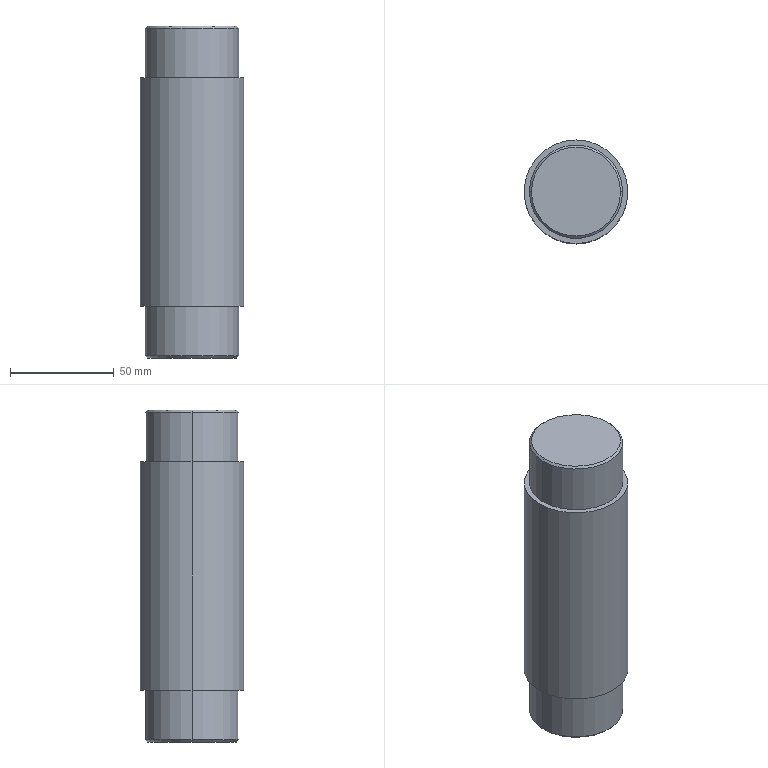Part | SolidWorks | features ICE 2, Chamfer 1, Extrusion 1 | 1 solid | 14 faces | box 50 x 50 x 160 mm | volume 295367 mm3 | cylinder 6 | cone 4 | plane 4 | commonest cylinder face diameters 45 x4 50 x2
STEP:
#1=CARTESIAN_POINT('',(-21.5,0.,-80.));
#2=VERTEX_POINT('',#1);
#3=CARTESIAN_POINT('',(21.5,0.,-80.));
#4=VERTEX_POINT('',#3);
#5=CARTESIAN_POINT('',(0.,0.,-80.));
#6=DIRECTION('',(0.,0.,-1.));
#7=DIRECTION('',(-1.,0.,0.));
#8=AXIS2_PLACEMENT_3D('',#5,#6,#7);
#9=CIRCLE('',#8,21.5);
#10=EDGE_CURVE('',#2,#4,#9,.T.);
#11=ORIENTED_EDGE('',*,*,#10,.F.);
#12=CARTESIAN_POINT('',(-22.5,0.,-79.));
#13=VERTEX_POINT('',#12);
#14=CARTESIAN_POINT('',(-21.5,0.,-80.));
#15=DIRECTION('',(-0.7071,0.,0.7071));
#16=VECTOR('',#15,1000.);
#17=LINE('',#14,#16);
#18=EDGE_CURVE('',#2,#13,#17,.T.);
#19=ORIENTED_EDGE('',*,*,#18,.T.);
#20=CARTESIAN_POINT('',(22.5,0.,-79.));
#21=VERTEX_POINT('',#20);
#22=CARTESIAN_POINT('',(0.,0.,-79.));
#23=DIRECTION('',(0.,0.,1.));
#24=DIRECTION('',(-1.,0.,0.));
#25=AXIS2_PLACEMENT_3D('',#22,#23,#24);
#26=CIRCLE('',#25,22.5);
#27=EDGE_CURVE('',#21,#13,#26,.T.);
#28=ORIENTED_EDGE('',*,*,#27,.F.);
#29=CARTESIAN_POINT('',(21.5,0.,-80.));
#30=DIRECTION('',(0.7071,0.,0.7071));
#31=VECTOR('',#30,1000.);
#32=LINE('',#29,#31);
#33=EDGE_CURVE('',#4,#21,#32,.T.);
#34=ORIENTED_EDGE('',*,*,#33,.F.);
#35=EDGE_LOOP('',(#11,#19,#28,#34));
#36=FACE_OUTER_BOUND('',#35,.T.);
#37=CARTESIAN_POINT('',(0.,0.,-80.));
#38=DIRECTION('',(0.,0.,1.));
#39=DIRECTION('',(1.,0.,0.));
#40=AXIS2_PLACEMENT_3D('',#37,#38,#39);
#41=CONICAL_SURFACE('',#40,21.5,0.7854);
#42=ADVANCED_FACE('',(#36),#41,.T.);
#43=CARTESIAN_POINT('',(21.5,0.,80.));
#44=VERTEX_POINT('',#43);
#45=CARTESIAN_POINT('',(-21.5,0.,80.));
#46=VERTEX_POINT('',#45);
#47=CARTESIAN_POINT('',(0.,0.,80.));
#48=DIRECTION('',(0.,0.,1.));
#49=DIRECTION('',(1.,0.,0.));
#50=AXIS2_PLACEMENT_3D('',#47,#48,#49);
#51=CIRCLE('',#50,21.5);
#52=EDGE_CURVE('',#44,#46,#51,.T.);
#53=ORIENTED_EDGE('',*,*,#52,.F.);
#54=CARTESIAN_POINT('',(22.5,0.,79.));
#55=VERTEX_POINT('',#54);
#56=CARTESIAN_POINT('',(21.5,0.,80.));
#57=DIRECTION('',(0.7071,0.,-0.7071));
#58=VECTOR('',#57,1000.);
#59=LINE('',#56,#58);
#60=EDGE_CURVE('',#44,#55,#59,.T.);
#61=ORIENTED_EDGE('',*,*,#60,.T.);
#62=CARTESIAN_POINT('',(-22.5,0.,79.));
#63=VERTEX_POINT('',#62);
#64=CARTESIAN_POINT('',(0.,0.,79.));
#65=DIRECTION('',(0.,0.,-1.));
#66=DIRECTION('',(1.,0.,0.));
#67=AXIS2_PLACEMENT_3D('',#64,#65,#66);
#68=CIRCLE('',#67,22.5);
#69=EDGE_CURVE('',#63,#55,#68,.T.);
#70=ORIENTED_EDGE('',*,*,#69,.F.);
#71=CARTESIAN_POINT('',(-21.5,0.,80.));
#72=DIRECTION('',(-0.7071,0.,-0.7071));
#73=VECTOR('',#72,1000.);
#74=LINE('',#71,#73);
#75=EDGE_CURVE('',#46,#63,#74,.T.);
#76=ORIENTED_EDGE('',*,*,#75,.F.);
#77=EDGE_LOOP('',(#53,#61,#70,#76));
#78=FACE_OUTER_BOUND('',#77,.T.);
#79=CARTESIAN_POINT('',(0.,0.,80.));
#80=DIRECTION('',(0.,0.,-1.));
#81=DIRECTION('',(-1.,0.,0.));
#82=AXIS2_PLACEMENT_3D('',#79,#80,#81);
#83=CONICAL_SURFACE('',#82,21.5,0.7854);
#84=ADVANCED_FACE('',(#78),#83,.T.);
#85=ORIENTED_EDGE('',*,*,#27,.T.);
#86=CARTESIAN_POINT('',(-22.5,0.,-55.));
#87=VERTEX_POINT('',#86);
#88=CARTESIAN_POINT('',(-22.5,0.,-80.));
#89=DIRECTION('',(0.,0.,1.));
#90=VECTOR('',#89,1000.);
#91=LINE('',#88,#90);
#92=EDGE_CURVE('',#13,#87,#91,.T.);
#93=ORIENTED_EDGE('',*,*,#92,.T.);
#94=CARTESIAN_POINT('',(22.5,0.,-55.));
#95=VERTEX_POINT('',#94);
#96=CARTESIAN_POINT('',(0.,0.,-55.));
#97=DIRECTION('',(0.,0.,-1.));
#98=DIRECTION('',(1.,0.,0.));
#99=AXIS2_PLACEMENT_3D('',#96,#97,#98);
#100=CIRCLE('',#99,22.5);
#101=EDGE_CURVE('',#87,#95,#100,.T.);
#102=ORIENTED_EDGE('',*,*,#101,.T.);
#103=CARTESIAN_POINT('',(22.5,0.,-80.));
#104=DIRECTION('',(0.,0.,1.));
#105=VECTOR('',#104,1000.);
#106=LINE('',#103,#105);
#107=EDGE_CURVE('',#21,#95,#106,.T.);
#108=ORIENTED_EDGE('',*,*,#107,.F.);
#109=EDGE_LOOP('',(#85,#93,#102,#108));
#110=FACE_OUTER_BOUND('',#109,.T.);
#111=CARTESIAN_POINT('',(0.,0.,-80.));
#112=DIRECTION('',(0.,0.,1.));
#113=DIRECTION('',(1.,0.,0.));
#114=AXIS2_PLACEMENT_3D('',#111,#112,#113);
#115=CYLINDRICAL_SURFACE('',#114,22.5);
#116=ADVANCED_FACE('',(#110),#115,.T.);
#117=ORIENTED_EDGE('',*,*,#69,.T.);
#118=CARTESIAN_POINT('',(22.5,0.,55.));
#119=VERTEX_POINT('',#118);
#120=CARTESIAN_POINT('',(22.5,0.,80.));
#121=DIRECTION('',(0.,0.,-1.));
#122=VECTOR('',#121,1000.);
#123=LINE('',#120,#122);
#124=EDGE_CURVE('',#55,#119,#123,.T.);
#125=ORIENTED_EDGE('',*,*,#124,.T.);
#126=CARTESIAN_POINT('',(-22.5,0.,55.));
#127=VERTEX_POINT('',#126);
#128=CARTESIAN_POINT('',(0.,0.,55.));
#129=DIRECTION('',(0.,0.,1.));
#130=DIRECTION('',(1.,0.,0.));
#131=AXIS2_PLACEMENT_3D('',#128,#129,#130);
#132=CIRCLE('',#131,22.5);
#133=EDGE_CURVE('',#119,#127,#132,.T.);
#134=ORIENTED_EDGE('',*,*,#133,.T.);
#135=CARTESIAN_POINT('',(-22.5,0.,80.));
#136=DIRECTION('',(0.,0.,-1.));
#137=VECTOR('',#136,1000.);
#138=LINE('',#135,#137);
#139=EDGE_CURVE('',#63,#127,#138,.T.);
#140=ORIENTED_EDGE('',*,*,#139,.F.);
#141=EDGE_LOOP('',(#117,#125,#134,#140));
#142=FACE_OUTER_BOUND('',#141,.T.);
#143=CARTESIAN_POINT('',(0.,0.,80.));
#144=DIRECTION('',(0.,0.,-1.));
#145=DIRECTION('',(-1.,0.,0.));
#146=AXIS2_PLACEMENT_3D('',#143,#144,#145);
#147=CYLINDRICAL_SURFACE('',#146,22.5);
#148=ADVANCED_FACE('',(#142),#147,.T.);
#149=CARTESIAN_POINT('',(25.,0.,55.));
#150=VERTEX_POINT('',#149);
#151=CARTESIAN_POINT('',(-25.,0.,55.));
#152=VERTEX_POINT('',#151);
#153=CARTESIAN_POINT('',(0.,0.,55.));
#154=DIRECTION('',(0.,0.,1.));
#155=DIRECTION('',(1.,0.,0.));
#156=AXIS2_PLACEMENT_3D('',#153,#154,#155);
#157=CIRCLE('',#156,25.);
#158=EDGE_CURVE('',#150,#152,#157,.T.);
#159=ORIENTED_EDGE('',*,*,#158,.F.);
#160=CARTESIAN_POINT('',(25.,0.,-55.));
#161=VERTEX_POINT('',#160);
#162=CARTESIAN_POINT('',(25.,0.,55.));
#163=DIRECTION('',(0.,0.,-1.));
#164=VECTOR('',#163,1000.);
#165=LINE('',#162,#164);
#166=EDGE_CURVE('',#150,#161,#165,.T.);
#167=ORIENTED_EDGE('',*,*,#166,.T.);
#168=CARTESIAN_POINT('',(-25.,0.,-55.));
#169=VERTEX_POINT('',#168);
#170=CARTESIAN_POINT('',(0.,0.,-55.));
#171=DIRECTION('',(0.,0.,1.));
#172=DIRECTION('',(1.,0.,0.));
#173=AXIS2_PLACEMENT_3D('',#170,#171,#172);
#174=CIRCLE('',#173,25.);
#175=EDGE_CURVE('',#161,#169,#174,.T.);
#176=ORIENTED_EDGE('',*,*,#175,.T.);
#177=CARTESIAN_POINT('',(-25.,0.,55.));
#178=DIRECTION('',(0.,0.,-1.));
#179=VECTOR('',#178,1000.);
#180=LINE('',#177,#179);
#181=EDGE_CURVE('',#152,#169,#180,.T.);
#182=ORIENTED_EDGE('',*,*,#181,.F.);
#183=EDGE_LOOP('',(#159,#167,#176,#182));
#184=FACE_OUTER_BOUND('',#183,.T.);
#185=CARTESIAN_POINT('',(0.,0.,55.));
#186=DIRECTION('',(0.,0.,-1.));
#187=DIRECTION('',(-1.,0.,0.));
#188=AXIS2_PLACEMENT_3D('',#185,#186,#187);
#189=CYLINDRICAL_SURFACE('',#188,25.);
#190=ADVANCED_FACE('',(#184),#189,.T.);
#191=ORIENTED_EDGE('',*,*,#166,.F.);
#192=CARTESIAN_POINT('',(0.,0.,55.));
#193=DIRECTION('',(0.,0.,1.));
#194=DIRECTION('',(1.,0.,0.));
#195=AXIS2_PLACEMENT_3D('',#192,#193,#194);
#196=CIRCLE('',#195,25.);
#197=EDGE_CURVE('',#152,#150,#196,.T.);
#198=ORIENTED_EDGE('',*,*,#197,.F.);
#199=ORIENTED_EDGE('',*,*,#181,.T.);
#200=CARTESIAN_POINT('',(0.,0.,-55.));
#201=DIRECTION('',(0.,0.,1.));
#202=DIRECTION('',(1.,0.,0.));
#203=AXIS2_PLACEMENT_3D('',#200,#201,#202);
#204=CIRCLE('',#203,25.);
#205=EDGE_CURVE('',#169,#161,#204,.T.);
#206=ORIENTED_EDGE('',*,*,#205,.T.);
#207=EDGE_LOOP('',(#191,#198,#199,#206));
#208=FACE_OUTER_BOUND('',#207,.T.);
#209=CARTESIAN_POINT('',(0.,0.,55.));
#210=DIRECTION('',(0.,0.,-1.));
#211=DIRECTION('',(-1.,0.,0.));
#212=AXIS2_PLACEMENT_3D('',#209,#210,#211);
#213=CYLINDRICAL_SURFACE('',#212,25.);
#214=ADVANCED_FACE('',(#208),#213,.T.);
#215=CARTESIAN_POINT('',(0.,0.,55.));
#216=DIRECTION('',(0.,0.,1.));
#217=DIRECTION('',(1.,0.,0.));
#218=AXIS2_PLACEMENT_3D('',#215,#216,#217);
#219=CIRCLE('',#218,22.5);
#220=EDGE_CURVE('',#127,#119,#219,.T.);
#221=ORIENTED_EDGE('',*,*,#220,.F.);
#222=ORIENTED_EDGE('',*,*,#133,.F.);
#223=EDGE_LOOP('',(#221,#222));
#224=FACE_BOUND('',#223,.T.);
#225=ORIENTED_EDGE('',*,*,#197,.T.);
#226=ORIENTED_EDGE('',*,*,#158,.T.);
#227=EDGE_LOOP('',(#225,#226));
#228=FACE_OUTER_BOUND('',#227,.T.);
#229=CARTESIAN_POINT('',(0.,0.,55.));
#230=DIRECTION('',(0.,0.,1.));
#231=DIRECTION('',(1.,0.,0.));
#232=AXIS2_PLACEMENT_3D('',#229,#230,#231);
#233=PLANE('',#232);
#234=ADVANCED_FACE('',(#224,#228),#233,.T.);
#235=CARTESIAN_POINT('',(0.,0.,-55.));
#236=DIRECTION('',(0.,0.,-1.));
#237=DIRECTION('',(1.,0.,0.));
#238=AXIS2_PLACEMENT_3D('',#235,#236,#237);
#239=CIRCLE('',#238,22.5);
#240=EDGE_CURVE('',#95,#87,#239,.T.);
#241=ORIENTED_EDGE('',*,*,#240,.F.);
#242=ORIENTED_EDGE('',*,*,#101,.F.);
#243=EDGE_LOOP('',(#241,#242));
#244=FACE_BOUND('',#243,.T.);
#245=ORIENTED_EDGE('',*,*,#205,.F.);
#246=ORIENTED_EDGE('',*,*,#175,.F.);
#247=EDGE_LOOP('',(#245,#246));
#248=FACE_OUTER_BOUND('',#247,.T.);
#249=CARTESIAN_POINT('',(0.,0.,-55.));
#250=DIRECTION('',(0.,0.,1.));
#251=DIRECTION('',(1.,0.,0.));
#252=AXIS2_PLACEMENT_3D('',#249,#250,#251);
#253=PLANE('',#252);
#254=ADVANCED_FACE('',(#244,#248),#253,.F.);
#255=ORIENTED_EDGE('',*,*,#124,.F.);
#256=CARTESIAN_POINT('',(0.,0.,79.));
#257=DIRECTION('',(0.,0.,-1.));
#258=DIRECTION('',(1.,0.,0.));
#259=AXIS2_PLACEMENT_3D('',#256,#257,#258);
#260=CIRCLE('',#259,22.5);
#261=EDGE_CURVE('',#55,#63,#260,.T.);
#262=ORIENTED_EDGE('',*,*,#261,.T.);
#263=ORIENTED_EDGE('',*,*,#139,.T.);
#264=ORIENTED_EDGE('',*,*,#220,.T.);
#265=EDGE_LOOP('',(#255,#262,#263,#264));
#266=FACE_OUTER_BOUND('',#265,.T.);
#267=CARTESIAN_POINT('',(0.,0.,80.));
#268=DIRECTION('',(0.,0.,-1.));
#269=DIRECTION('',(-1.,0.,0.));
#270=AXIS2_PLACEMENT_3D('',#267,#268,#269);
#271=CYLINDRICAL_SURFACE('',#270,22.5);
#272=ADVANCED_FACE('',(#266),#271,.T.);
#273=CARTESIAN_POINT('',(0.,0.,80.));
#274=DIRECTION('',(0.,0.,1.));
#275=DIRECTION('',(1.,0.,0.));
#276=AXIS2_PLACEMENT_3D('',#273,#274,#275);
#277=CIRCLE('',#276,21.5);
#278=EDGE_CURVE('',#46,#44,#277,.T.);
#279=ORIENTED_EDGE('',*,*,#278,.T.);
#280=ORIENTED_EDGE('',*,*,#52,.T.);
#281=EDGE_LOOP('',(#279,#280));
#282=FACE_OUTER_BOUND('',#281,.T.);
#283=CARTESIAN_POINT('',(0.,0.,80.));
#284=DIRECTION('',(0.,0.,1.));
#285=DIRECTION('',(1.,0.,0.));
#286=AXIS2_PLACEMENT_3D('',#283,#284,#285);
#287=PLANE('',#286);
#288=ADVANCED_FACE('',(#282),#287,.T.);
#289=ORIENTED_EDGE('',*,*,#92,.F.);
#290=CARTESIAN_POINT('',(0.,0.,-79.));
#291=DIRECTION('',(0.,0.,1.));
#292=DIRECTION('',(-1.,0.,0.));
#293=AXIS2_PLACEMENT_3D('',#290,#291,#292);
#294=CIRCLE('',#293,22.5);
#295=EDGE_CURVE('',#13,#21,#294,.T.);
#296=ORIENTED_EDGE('',*,*,#295,.T.);
#297=ORIENTED_EDGE('',*,*,#107,.T.);
#298=ORIENTED_EDGE('',*,*,#240,.T.);
#299=EDGE_LOOP('',(#289,#296,#297,#298));
#300=FACE_OUTER_BOUND('',#299,.T.);
#301=CARTESIAN_POINT('',(0.,0.,-80.));
#302=DIRECTION('',(0.,0.,1.));
#303=DIRECTION('',(1.,0.,0.));
#304=AXIS2_PLACEMENT_3D('',#301,#302,#303);
#305=CYLINDRICAL_SURFACE('',#304,22.5);
#306=ADVANCED_FACE('',(#300),#305,.T.);
#307=CARTESIAN_POINT('',(0.,0.,-80.));
#308=DIRECTION('',(0.,0.,-1.));
#309=DIRECTION('',(-1.,0.,0.));
#310=AXIS2_PLACEMENT_3D('',#307,#308,#309);
#311=CIRCLE('',#310,21.5);
#312=EDGE_CURVE('',#4,#2,#311,.T.);
#313=ORIENTED_EDGE('',*,*,#312,.T.);
#314=ORIENTED_EDGE('',*,*,#10,.T.);
#315=EDGE_LOOP('',(#313,#314));
#316=FACE_OUTER_BOUND('',#315,.T.);
#317=CARTESIAN_POINT('',(0.,0.,-80.));
#318=DIRECTION('',(0.,0.,-1.));
#319=DIRECTION('',(-1.,0.,0.));
#320=AXIS2_PLACEMENT_3D('',#317,#318,#319);
#321=PLANE('',#320);
#322=ADVANCED_FACE('',(#316),#321,.T.);
#323=ORIENTED_EDGE('',*,*,#60,.F.);
#324=ORIENTED_EDGE('',*,*,#278,.F.);
#325=ORIENTED_EDGE('',*,*,#75,.T.);
#326=ORIENTED_EDGE('',*,*,#261,.F.);
#327=EDGE_LOOP('',(#323,#324,#325,#326));
#328=FACE_OUTER_BOUND('',#327,.T.);
#329=CARTESIAN_POINT('',(0.,0.,80.));
#330=DIRECTION('',(0.,0.,-1.));
#331=DIRECTION('',(-1.,0.,0.));
#332=AXIS2_PLACEMENT_3D('',#329,#330,#331);
#333=CONICAL_SURFACE('',#332,21.5,0.7854);
#334=ADVANCED_FACE('',(#328),#333,.T.);
#335=ORIENTED_EDGE('',*,*,#18,.F.);
#336=ORIENTED_EDGE('',*,*,#312,.F.);
#337=ORIENTED_EDGE('',*,*,#33,.T.);
#338=ORIENTED_EDGE('',*,*,#295,.F.);
#339=EDGE_LOOP('',(#335,#336,#337,#338));
#340=FACE_OUTER_BOUND('',#339,.T.);
#341=CARTESIAN_POINT('',(0.,0.,-80.));
#342=DIRECTION('',(0.,0.,1.));
#343=DIRECTION('',(1.,0.,0.));
#344=AXIS2_PLACEMENT_3D('',#341,#342,#343);
#345=CONICAL_SURFACE('',#344,21.5,0.7854);
#346=ADVANCED_FACE('',(#340),#345,.T.);
#347=CLOSED_SHELL('',(#42,#84,#116,#148,#190,#214,#234,#254,#272,#288,#306,#322,#334,#346));
#348=MANIFOLD_SOLID_BREP('',#347);
#349=CARTESIAN_POINT('',(0.,0.,0.));
#350=DIRECTION('',(0.,0.,1.));
#351=DIRECTION('',(1.,0.,0.));
#352=AXIS2_PLACEMENT_3D('',#349,#350,#351);
#353=(LENGTH_UNIT()NAMED_UNIT(*)SI_UNIT(.MILLI.,.METRE.));
#354=UNCERTAINTY_MEASURE_WITH_UNIT(LENGTH_MEASURE(0.00001),#353,'','');
#355=(NAMED_UNIT(*)PLANE_ANGLE_UNIT()SI_UNIT($,.RADIAN.));
#356=(NAMED_UNIT(*)SI_UNIT($,.STERADIAN.)SOLID_ANGLE_UNIT());
#357=(GEOMETRIC_REPRESENTATION_CONTEXT(3)GLOBAL_UNCERTAINTY_ASSIGNED_CONTEXT((#354))GLOBAL_UNIT_ASSIGNED_CONTEXT((#353,#355,#356))REPRESENTATION_CONTEXT('',''));
#358=ADVANCED_BREP_SHAPE_REPRESENTATION('',(#348,#352),#357);